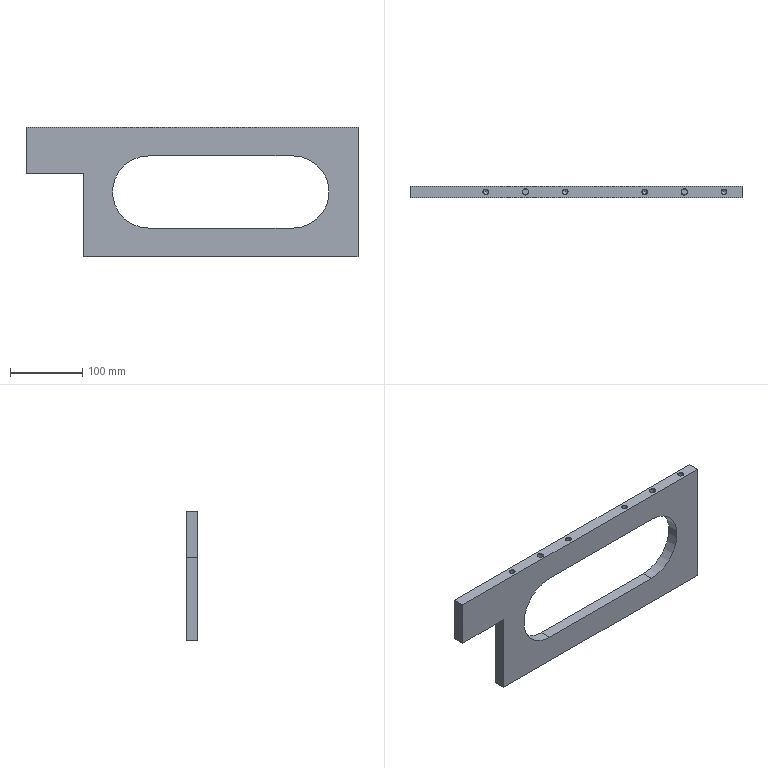Part | STEP file | Tube feed_id1830_x_t | 1 solid | 46 faces | box 460 x 16 x 180 mm | volume 718962 mm3 | cone 18 | plane 14 | cylinder 14 | commonest cylinder face diameters 6.8 x8 8 x4 100 x2